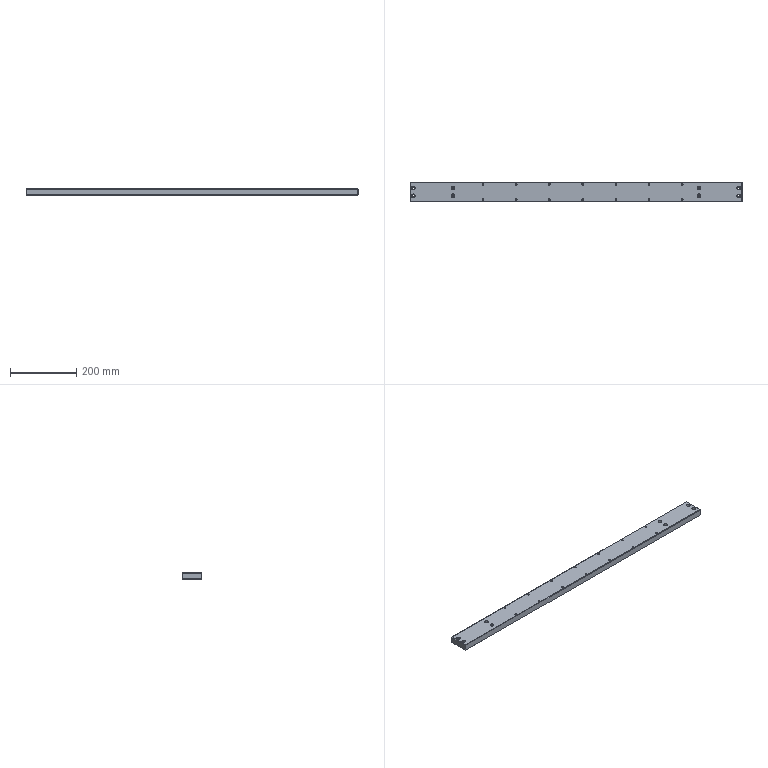Part | SolidWorks | features Chamfer 2, HoleWzd 2, Extrusion 1, LPattern 1 | 1 solid | 114 faces | box 1000 x 60 x 20 mm | volume 1185060 mm3 | cylinder 60 | cone 28 | plane 26 | commonest cylinder face diameters 5 x28 6.5 x16 11 x16